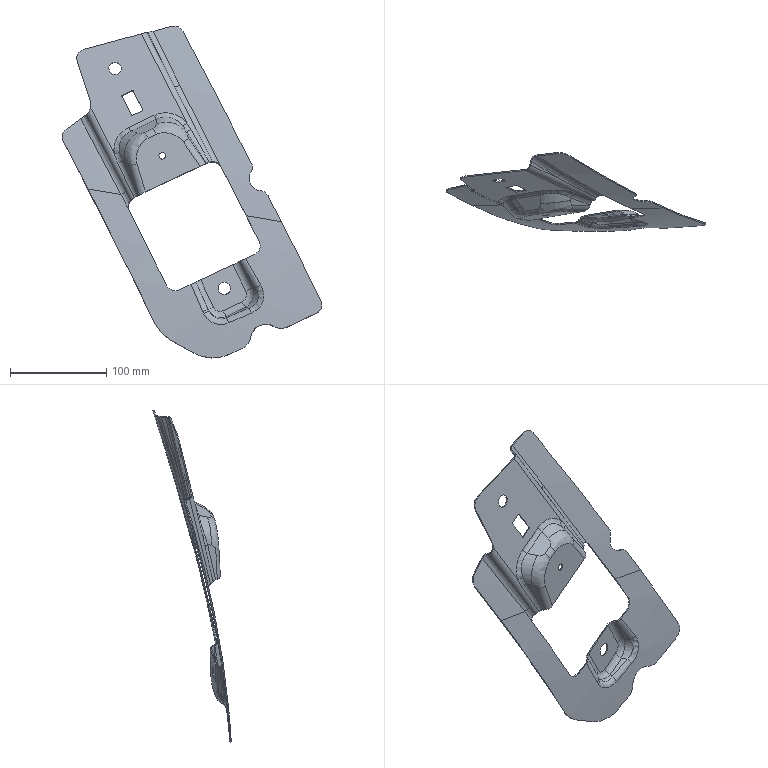Part | STEP file | FNA5401831 | 1 solid | 165 faces | box 269.629 x 81.435 x 345.025 mm | volume 52905 mm3 | spline 119 | cylinder 34 | plane 10 | other 2 | commonest cylinder face diameters 16 x5 2 x4 13 x4 14 x3 18.4 x3 7 x2